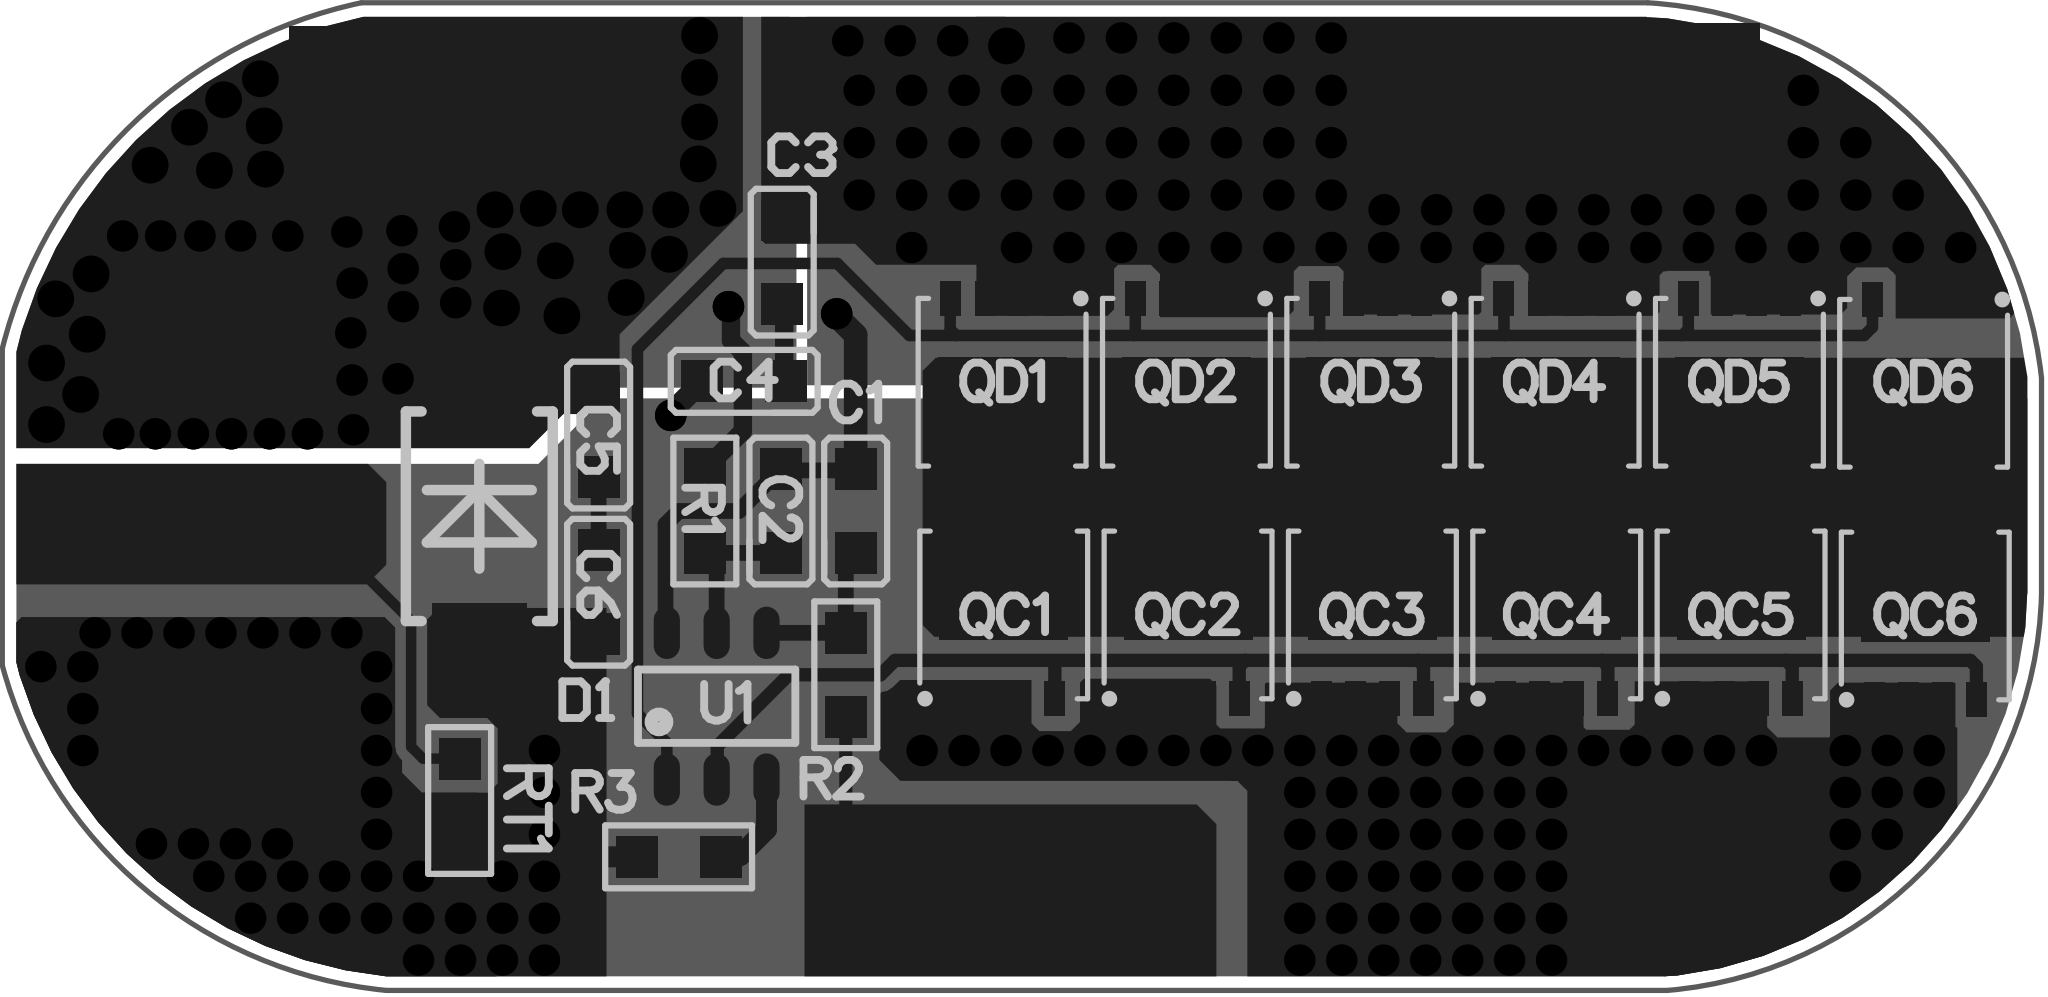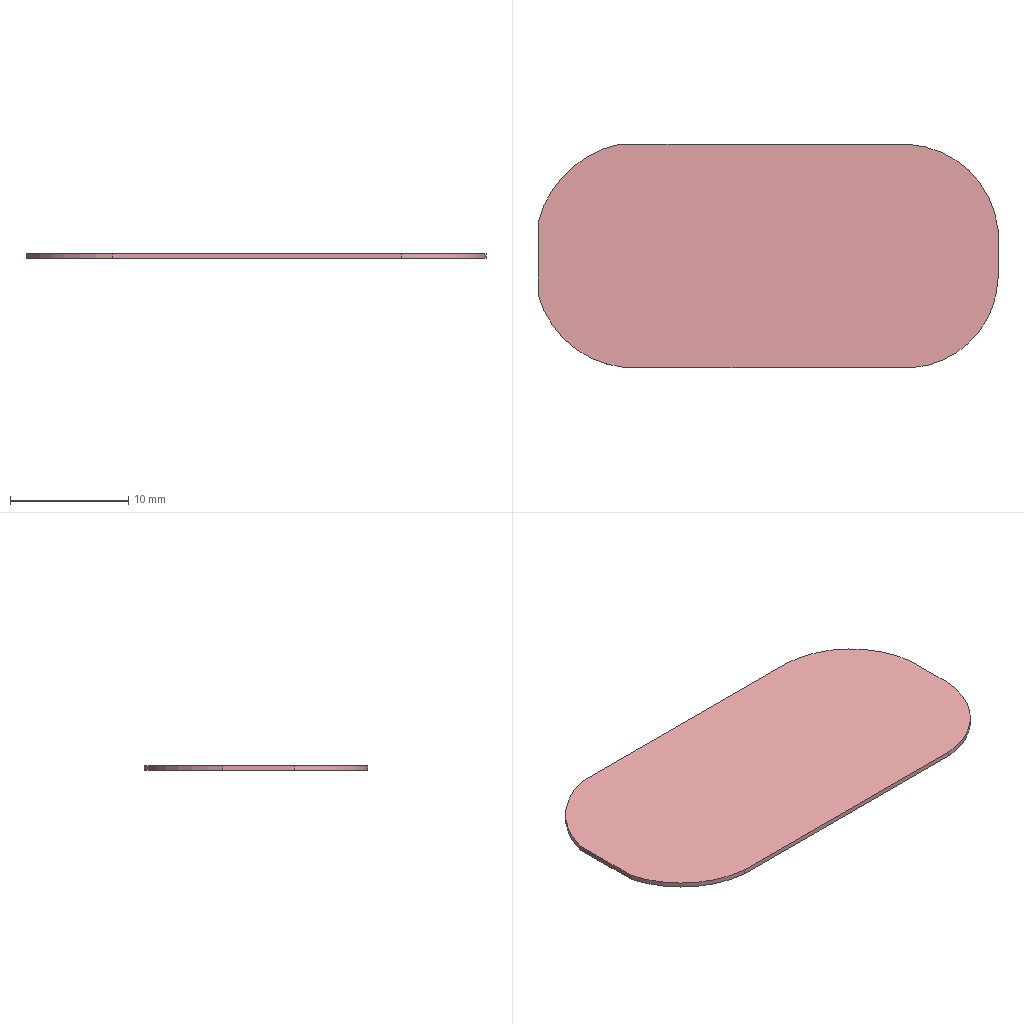Circuit board layout | Altium Designer | box 38.9 x 18.8 x 0.4 mm
Layer stack:
# Altium Designer layer stack of  (unit mm; dielectric type: 0 none, 1 core, 2 prepreg, 3 surface material)
index,name,kind,layer,copper_thickness_mm,dielectric_type,dielectric_thickness_mm,dielectric_material,dielectric_constant
0,Top Paste,other,,,,,,
1,Top Overlay,other,,,,,,
2,Top Solder,dielectric,,,3,0.0102,Solder Resist,3.5
3,Top Layer,copper,Top Layer,0.0356,,,,
4,Dielectric 1,dielectric,,,0,0.32,FR-4,4.8
5,Bottom Layer,copper,Bottom Layer,0.0356,,,,
6,Bottom Solder,dielectric,,,3,0.0102,Solder Resist,3.5
7,Bottom Overlay,other,,,,,,
8,Bottom Paste,other,,,,,,
# drill layer pairs: low layer,high layer
drill_pair,Top Layer,Bottom Layer
Part placement:
Designator,Comment,Layer,Footprint,Center-X(mm),Center-Y(mm),Rotation
P-,Pad,TopLayer,Pad10X8mm,-2.623,-14.05,0
T,Pad,TopLayer,Pad10X8mm,-2.673,-10.025,90
P-,Pad,TopLayer,Pad10X8mm,25.152,-16.475,90
P+,Pad,TopLayer,Pad10X8mm,-2.667,-6.337,0
D1,RS2M,TopLayer,SMA(DO-214AC),2.25,-9.8,0
C6,0.1uF,TopLayer,C0603A,4.525,-11.25,270
C5,0.1uF,TopLayer,C0603A,4.525,-8.25,270
C4,0.1uF,TopLayer,C0603A,7.3,-7.225,0
C3,0.1uF,TopLayer,C0603A,8.025,-4.95,90
BM,Pad,TopLayer,Pad10X8mm,12.252,-17.025,0
B-,Pad,TopLayer,Pad10X8mm,23.152,-1.9,0
B+,Pad,TopLayer,Pad10X8mm,2.127,-1.95,0
QC6,N MOS*,TopLayer,DFN-3x3L8(T3P),29.816,-11.703,0
QD6,N MOS*,TopLayer,DFN-3x3L8(T3P),29.785,-7.262,180
RT1,10K,TopLayer,R0603A,1.875,-15.225,90
QD5,N MOS*,TopLayer,DFN-3x3L8(T3P),26.274,-7.242,180
QD4,N MOS*,TopLayer,DFN-3x3L8(T3P),22.76,-7.242,180
QD3,N MOS*,TopLayer,DFN-3x3L8(T3P),19.245,-7.242,180
QD2,N MOS*,TopLayer,DFN-3x3L8(T3P),15.731,-7.242,180
QC5,N MOS*,TopLayer,DFN-3x3L8(T3P),26.305,-11.683,0
QC4,N MOS*,TopLayer,DFN-3x3L8(T3P),22.791,-11.683,0
QC3,N MOS*,TopLayer,DFN-3x3L8(T3P),19.276,-11.683,0
QC2,N MOS*,TopLayer,DFN-3x3L8(T3P),15.762,-11.683,0
QC1,N MOS*,TopLayer,DFN-3x3L8(T3P),12.248,-11.683,0
U1,CW1025*,TopLayer,SOT23-6A,6.775,-13.425,90
R3,2.2K,TopLayer,R0603A,6.05,-16.3,0
R2,330R,TopLayer,R0603A,9.237,-12.825,90
R1,330R,TopLayer,R0603A,6.55,-9.7,270
QD1,N MOS*,TopLayer,DFN-3x3L8(T3P),12.217,-7.242,180
C2,0.1uF,TopLayer,C0603A,8,-9.7,270
C1,0.1uF,TopLayer,C0603A,9.425,-9.7,270
Pad and via stacks:
# Altium Designer via and pad stacks of  (unit mm). Each distinct definition once, with the count of objects using it.
# via: kind,start_layer,end_layer,hole_mm,diameter_mm,mode(0 simple;1 top-mid-bottom;2 full stack),diameter_per_layer,count,example_net
# pad: kind,layer,hole_mm,hole_type(0 round;1 square;2 slot),plating,top_size,top_shape(1 round;2 rect;3 octagon;9 rounded rect),mid_size,bottom_size,mode,footprint,size_per_layer,count,example
pad,Keep-Out Layer,0.0635,0,plated,0.0635x0.0635,1,0.0635x0.0635,0.0635x0.0635,0,,,16,1
pad,Top Layer,0,0,plated,1.8x1.6,2,1.8x1.6,1.8x1.6,0,SMA(DO-214AC),,2,D1.1
pad,Top Layer,0,0,plated,0.8x0.8,2,0.8x0.8,0.8x0.8,0,C0603A,,12,C3.1
pad,Top Layer,0,0,plated,0.8x0.8,2,0.8x0.8,0.8x0.8,0,R0603A,,8,R3.2
pad,Top Layer,0,2,plated,7x3,2,7x3,7x3,0,Pad10X8mm,,3,BM.1
pad,Top Layer,0,2,plated,4x3,2,4x3,4x3,0,Pad10X8mm,,2,P-.1
pad,Top Layer,0,2,plated,2x4,2,2x4,2x4,0,Pad10X8mm,,1,T.1
pad,Top Layer,0,2,plated,3x4,2,3x4,3x4,0,Pad10X8mm,,1,P-.1
pad,Top Layer,0,0,plated,1x0.5,1,1x0.5,1x0.5,0,SOT23-6A,,6,U1.1
pad,Top Layer,0,0,plated,0.4x0.65,2,0.4x0.65,0.4x0.65,0,DFN-3x3L8(T3P),,96,QD6.1
pad,Top Layer,0,0,plated,2.45x1.76,2,2.45x1.76,2.45x1.76,0,DFN-3x3L8(T3P),,12,QD6.3
via,Top Layer,Bottom Layer,0.4,0.6,0,,207,B+
via,Top Layer,Bottom Layer,0.5,0.7,0,,31,B+
Copper pours:
name,layer,net,type(0 solid;1 hatched;2 none)
NONET_L-01_P-001,Top Layer,B+,0
NONET_L-01_P-001,Top Layer,P-,0
NONET_L-01_P-001,Top Layer,B-,0
NONET_L-01_P-001,Top Layer,B-,0
NONET_L-01_P-001,Top Layer,B-,0
NONET_L-01_P-001,Top Layer,P-,0
NONET_L-01_P-001,Top Layer,P-,0
NONET_L-01_P-001,Top Layer,P-,0
NONET_L-01_P-001,Top Layer,NetQC1_3,0
NONET_L-01_P-001,Top Layer,BM,0
NONET_L-01_P-001,Top Layer,T,0
NONET_L-01_P-001,Bottom Layer,P-,0
NONET_L-01_P-001,Bottom Layer,B+,0
NONET_L-01_P-001,Bottom Layer,B-,0
Design rules, without the lines most boards share:
# Altium Designer design rules of  (exported by Altium Designer, unit mm)
# columns: name | kind | enabled | priority | scope1 | scope2 | descriptor | typed fields (field=value)
Schematic Supply Nets | 41 | enabled | 1 | InNet('P-') | All | Supply Net(s)(InNet('P-')) |
NetAntennae | 56 | enabled | 1 | All | All | Net Antennae (Tolerance=0mm) (All) |
SilkToSilkClearance | 55 | enabled | 1 | All | All | Silk to Silk (Clearance=0.254mm) (All),(All) |
SilkToSolderMaskClearance | 54 | enabled | 1 | IsPad | All | Silk To Solder Mask (Clearance=0.254mm) (IsPad),(All) |
MinimumSolderMaskSliver | 53 | enabled | 1 | All | All | Minimum Solder Mask Sliver (Gap=0.254mm) (All),(All) |
HoleToHoleClearance | 52 | enabled | 1 | All | All | Hole To Hole Clearance (Gap=0.254mm) (All),(All) | gap=0.254
DiffPairsRouting | 51 | enabled | 1 | All | All | Differential Pairs Uncoupled Length using the Gap Constraints (Min=0.254mm) (Max=0.254mm) (Prefered=0.254mm)  and Width Constraints (Min=0.381mm) (Max=0.381mm) (Prefered=0.381mm) (All) |
HoleSize | 42 | enabled | 1 | All | All | Hole Size Constraint (Min=0.025mm) (Max=2.54mm) (All) |
Height | 50 | enabled | 1 | All | All | Height Constraint (Min=0mm) (Max=25.4mm) (Prefered=12.7mm) (All) | min_height=0 max_height=25.4
ComponentClearance | 24 | enabled | 1 | All | All | Component Clearance Constraint ( Horizontal Gap = 0.2mm, Vertical Gap = 0.254mm ) (All),(All)  | gap=0.2
SolderMaskExpansion | 13 | enabled | 1 | All | All | Solder Mask Expansion (Expansion =0.102mm) (All) | expansion=0.1016
PasteMaskExpansion | 14 | enabled | 1 | All | All | Paste Mask Expansion (Expansion =0mm) (All) | expansion=0
RoutingVias | 11 | enabled | 1 | All | All | Routing Via (MinHoleWidth=0.3mm) (MaxHoleWidth=0.3mm) (PreferredHoleWidth=0.3mm) (MinWidth=0.5mm) (MaxWidth=0.5mm) (PreferedWidth=0.5mm) (All) | via_min_hole=0.3 via_max_hole=0.3 via_preferred_diameter=0.5 via_preferred_hole=0.3
RoutingCorners | 10 | enabled | 1 | All | All | Routing Corners (Style=45-Degree) (Min Setback=2.54mm) (Max Setback=2.54mm) (All) |
Width | 2 | enabled | 1 | All | All | Width Constraint (Min=0.15mm) (Max=1mm) (Preferred=0.2mm) (All) |
PolygonConnect | 20 | enabled | 1 | All | All | Polygon Connect Rule(Direct Connect )(Conductor Width=0.254mm) (Relief Angle=90 Angle) (Entries=4) (Air Gap Width=0.254mm) (All),(All) | connect_style(0=relief,1=direct,2=none)=1 relief_conductor_width=0.254 relief_entries=4
PlaneClearance | 12 | enabled | 1 | All | All | Power Plane Clearance (Clearance =0.508mm) (All) | clearance=0.508
PlaneConnect | 6 | enabled | 1 | All | All | Power Plane Connect Rule(Relief Connect )(Expansion=0.508mm) (Conductor Width=0.254mm) (Air Gap=0.254mm) (Entries=4) (All) | relief_conductor_width=0.254 relief_entries=4 relief_expansion=0.508
Clearance | 0 | enabled | 1 | All | All | Clearance Constraint (Gap=0.2mm) (All),(All) | gap=0.2